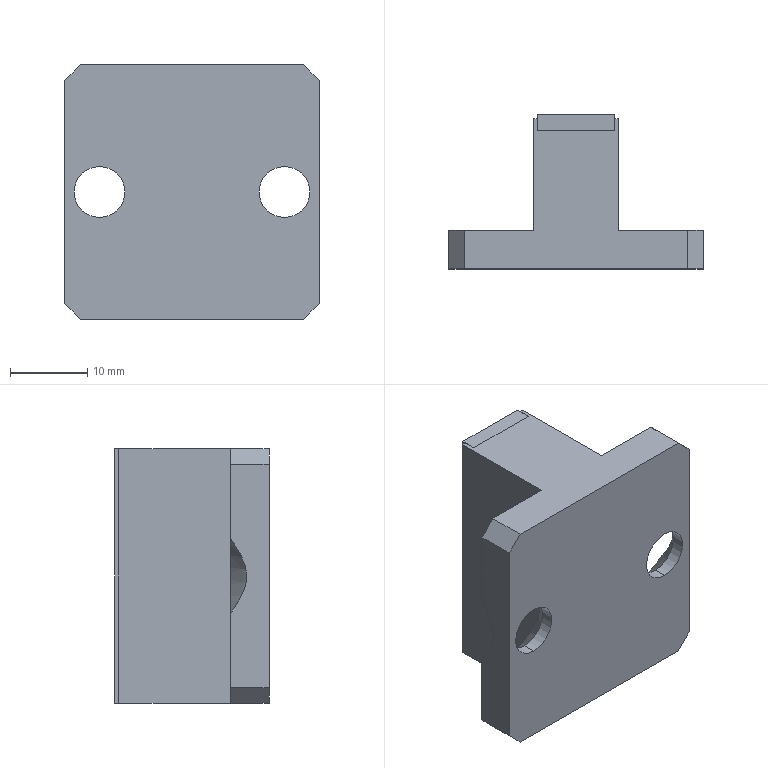Part | SolidWorks | features ICE 2, Chamfer 1, Extrusion 1, HoleWzd 1 | 2 solids | 36 faces | box 33 x 20 x 33 mm | volume 10213 mm3 | plane 28 | cylinder 4 | cone 4 | commonest cylinder face diameters 6.6 x4
STEP:
#1=CARTESIAN_POINT('',(-5.,18.,-16.5));
#2=VERTEX_POINT('',#1);
#3=CARTESIAN_POINT('',(-5.,18.,16.5));
#4=VERTEX_POINT('',#3);
#5=CARTESIAN_POINT('',(-5.,18.,-16.5));
#6=DIRECTION('',(0.,0.,1.));
#7=VECTOR('',#6,1000.);
#8=LINE('',#5,#7);
#9=EDGE_CURVE('',#2,#4,#8,.T.);
#10=ORIENTED_EDGE('',*,*,#9,.T.);
#11=CARTESIAN_POINT('',(-5.,20.,16.5));
#12=VERTEX_POINT('',#11);
#13=CARTESIAN_POINT('',(-5.,20.,16.5));
#14=DIRECTION('',(0.,-1.,0.));
#15=VECTOR('',#14,1000.);
#16=LINE('',#13,#15);
#17=EDGE_CURVE('',#12,#4,#16,.T.);
#18=ORIENTED_EDGE('',*,*,#17,.F.);
#19=CARTESIAN_POINT('',(-5.,20.,-16.5));
#20=VERTEX_POINT('',#19);
#21=CARTESIAN_POINT('',(-5.,20.,-16.5));
#22=DIRECTION('',(0.,0.,1.));
#23=VECTOR('',#22,1000.);
#24=LINE('',#21,#23);
#25=EDGE_CURVE('',#20,#12,#24,.T.);
#26=ORIENTED_EDGE('',*,*,#25,.F.);
#27=CARTESIAN_POINT('',(-5.,20.,-16.5));
#28=DIRECTION('',(0.,-1.,0.));
#29=VECTOR('',#28,1000.);
#30=LINE('',#27,#29);
#31=EDGE_CURVE('',#20,#2,#30,.T.);
#32=ORIENTED_EDGE('',*,*,#31,.T.);
#33=EDGE_LOOP('',(#10,#18,#26,#32));
#34=FACE_OUTER_BOUND('',#33,.T.);
#35=CARTESIAN_POINT('',(-5.,20.,-16.5));
#36=DIRECTION('',(1.,0.,0.));
#37=DIRECTION('',(0.,0.,-1.));
#38=AXIS2_PLACEMENT_3D('',#35,#36,#37);
#39=PLANE('',#38);
#40=ADVANCED_FACE('',(#34),#39,.F.);
#41=CARTESIAN_POINT('',(5.,18.,16.5));
#42=VERTEX_POINT('',#41);
#43=CARTESIAN_POINT('',(-5.,18.,16.5));
#44=DIRECTION('',(1.,0.,0.));
#45=VECTOR('',#44,1000.);
#46=LINE('',#43,#45);
#47=EDGE_CURVE('',#4,#42,#46,.T.);
#48=ORIENTED_EDGE('',*,*,#47,.T.);
#49=CARTESIAN_POINT('',(5.,20.,16.5));
#50=VERTEX_POINT('',#49);
#51=CARTESIAN_POINT('',(5.,20.,16.5));
#52=DIRECTION('',(0.,-1.,0.));
#53=VECTOR('',#52,1000.);
#54=LINE('',#51,#53);
#55=EDGE_CURVE('',#50,#42,#54,.T.);
#56=ORIENTED_EDGE('',*,*,#55,.F.);
#57=CARTESIAN_POINT('',(-5.,20.,16.5));
#58=DIRECTION('',(1.,0.,0.));
#59=VECTOR('',#58,1000.);
#60=LINE('',#57,#59);
#61=EDGE_CURVE('',#12,#50,#60,.T.);
#62=ORIENTED_EDGE('',*,*,#61,.F.);
#63=ORIENTED_EDGE('',*,*,#17,.T.);
#64=EDGE_LOOP('',(#48,#56,#62,#63));
#65=FACE_OUTER_BOUND('',#64,.T.);
#66=CARTESIAN_POINT('',(-5.,20.,16.5));
#67=DIRECTION('',(0.,0.,-1.));
#68=DIRECTION('',(-1.,0.,0.));
#69=AXIS2_PLACEMENT_3D('',#66,#67,#68);
#70=PLANE('',#69);
#71=ADVANCED_FACE('',(#65),#70,.F.);
#72=CARTESIAN_POINT('',(5.,18.,-16.5));
#73=VERTEX_POINT('',#72);
#74=CARTESIAN_POINT('',(5.,18.,-16.5));
#75=DIRECTION('',(0.,0.,-1.));
#76=VECTOR('',#75,1000.);
#77=LINE('',#74,#76);
#78=EDGE_CURVE('',#42,#73,#77,.T.);
#79=ORIENTED_EDGE('',*,*,#78,.T.);
#80=CARTESIAN_POINT('',(5.,20.,-16.5));
#81=VERTEX_POINT('',#80);
#82=CARTESIAN_POINT('',(5.,20.,-16.5));
#83=DIRECTION('',(0.,-1.,0.));
#84=VECTOR('',#83,1000.);
#85=LINE('',#82,#84);
#86=EDGE_CURVE('',#81,#73,#85,.T.);
#87=ORIENTED_EDGE('',*,*,#86,.F.);
#88=CARTESIAN_POINT('',(5.,20.,-16.5));
#89=DIRECTION('',(0.,0.,-1.));
#90=VECTOR('',#89,1000.);
#91=LINE('',#88,#90);
#92=EDGE_CURVE('',#50,#81,#91,.T.);
#93=ORIENTED_EDGE('',*,*,#92,.F.);
#94=ORIENTED_EDGE('',*,*,#55,.T.);
#95=EDGE_LOOP('',(#79,#87,#93,#94));
#96=FACE_OUTER_BOUND('',#95,.T.);
#97=CARTESIAN_POINT('',(5.,20.,-16.5));
#98=DIRECTION('',(-1.,0.,0.));
#99=DIRECTION('',(0.,0.,1.));
#100=AXIS2_PLACEMENT_3D('',#97,#98,#99);
#101=PLANE('',#100);
#102=ADVANCED_FACE('',(#96),#101,.F.);
#103=CARTESIAN_POINT('',(-5.,18.,-16.5));
#104=DIRECTION('',(-1.,0.,0.));
#105=VECTOR('',#104,1000.);
#106=LINE('',#103,#105);
#107=EDGE_CURVE('',#73,#2,#106,.T.);
#108=ORIENTED_EDGE('',*,*,#107,.T.);
#109=ORIENTED_EDGE('',*,*,#31,.F.);
#110=CARTESIAN_POINT('',(-5.,20.,-16.5));
#111=DIRECTION('',(-1.,0.,0.));
#112=VECTOR('',#111,1000.);
#113=LINE('',#110,#112);
#114=EDGE_CURVE('',#81,#20,#113,.T.);
#115=ORIENTED_EDGE('',*,*,#114,.F.);
#116=ORIENTED_EDGE('',*,*,#86,.T.);
#117=EDGE_LOOP('',(#108,#109,#115,#116));
#118=FACE_OUTER_BOUND('',#117,.T.);
#119=CARTESIAN_POINT('',(-5.,20.,-16.5));
#120=DIRECTION('',(0.,0.,1.));
#121=DIRECTION('',(1.,0.,0.));
#122=AXIS2_PLACEMENT_3D('',#119,#120,#121);
#123=PLANE('',#122);
#124=ADVANCED_FACE('',(#118),#123,.F.);
#125=ORIENTED_EDGE('',*,*,#25,.T.);
#126=ORIENTED_EDGE('',*,*,#61,.T.);
#127=ORIENTED_EDGE('',*,*,#92,.T.);
#128=ORIENTED_EDGE('',*,*,#114,.T.);
#129=EDGE_LOOP('',(#125,#126,#127,#128));
#130=FACE_OUTER_BOUND('',#129,.T.);
#131=CARTESIAN_POINT('',(-5.,20.,16.5));
#132=DIRECTION('',(0.,1.,0.));
#133=DIRECTION('',(0.,0.,1.));
#134=AXIS2_PLACEMENT_3D('',#131,#132,#133);
#135=PLANE('',#134);
#136=ADVANCED_FACE('',(#130),#135,.T.);
#137=ORIENTED_EDGE('',*,*,#9,.F.);
#138=ORIENTED_EDGE('',*,*,#107,.F.);
#139=ORIENTED_EDGE('',*,*,#78,.F.);
#140=ORIENTED_EDGE('',*,*,#47,.F.);
#141=EDGE_LOOP('',(#137,#138,#139,#140));
#142=FACE_OUTER_BOUND('',#141,.T.);
#143=CARTESIAN_POINT('',(-5.,18.,16.5));
#144=DIRECTION('',(0.,1.,0.));
#145=DIRECTION('',(0.,0.,1.));
#146=AXIS2_PLACEMENT_3D('',#143,#144,#145);
#147=PLANE('',#146);
#148=ADVANCED_FACE('',(#142),#147,.F.);
#149=CLOSED_SHELL('',(#40,#71,#102,#124,#136,#148));
#150=MANIFOLD_SOLID_BREP('',#149);
#151=CARTESIAN_POINT('',(-12.,0.,-3.3));
#152=VERTEX_POINT('',#151);
#153=CARTESIAN_POINT('',(-12.,0.,3.3));
#154=VERTEX_POINT('',#153);
#155=CARTESIAN_POINT('',(-12.,0.,0.));
#156=DIRECTION('',(0.,1.,0.));
#157=DIRECTION('',(0.,0.,1.));
#158=AXIS2_PLACEMENT_3D('',#155,#156,#157);
#159=CIRCLE('',#158,3.3);
#160=EDGE_CURVE('',#152,#154,#159,.T.);
#161=ORIENTED_EDGE('',*,*,#160,.F.);
#162=CARTESIAN_POINT('',(-12.,1.7,-3.3));
#163=VERTEX_POINT('',#162);
#164=CARTESIAN_POINT('',(-12.,5.,-3.3));
#165=DIRECTION('',(0.,1.,0.));
#166=VECTOR('',#165,1000.);
#167=LINE('',#164,#166);
#168=EDGE_CURVE('',#152,#163,#167,.T.);
#169=ORIENTED_EDGE('',*,*,#168,.T.);
#170=CARTESIAN_POINT('',(-12.,1.7,3.3));
#171=VERTEX_POINT('',#170);
#172=CARTESIAN_POINT('',(-12.,1.7,0.));
#173=DIRECTION('',(0.,1.,0.));
#174=DIRECTION('',(0.,0.,1.));
#175=AXIS2_PLACEMENT_3D('',#172,#173,#174);
#176=CIRCLE('',#175,3.3);
#177=EDGE_CURVE('',#163,#171,#176,.T.);
#178=ORIENTED_EDGE('',*,*,#177,.T.);
#179=CARTESIAN_POINT('',(-12.,5.,3.3));
#180=DIRECTION('',(0.,1.,0.));
#181=VECTOR('',#180,1000.);
#182=LINE('',#179,#181);
#183=EDGE_CURVE('',#154,#171,#182,.T.);
#184=ORIENTED_EDGE('',*,*,#183,.F.);
#185=EDGE_LOOP('',(#161,#169,#178,#184));
#186=FACE_OUTER_BOUND('',#185,.T.);
#187=CARTESIAN_POINT('',(-12.,5.,0.));
#188=DIRECTION('',(0.,1.,0.));
#189=DIRECTION('',(0.,0.,1.));
#190=AXIS2_PLACEMENT_3D('',#187,#188,#189);
#191=CYLINDRICAL_SURFACE('',#190,3.3);
#192=ADVANCED_FACE('',(#186),#191,.F.);
#193=ORIENTED_EDGE('',*,*,#177,.F.);
#194=CARTESIAN_POINT('',(-12.,5.,-6.6));
#195=VERTEX_POINT('',#194);
#196=CARTESIAN_POINT('',(-12.,5.,-6.6));
#197=DIRECTION('',(0.,0.7071,-0.7071));
#198=VECTOR('',#197,1000.);
#199=LINE('',#196,#198);
#200=EDGE_CURVE('',#163,#195,#199,.T.);
#201=ORIENTED_EDGE('',*,*,#200,.T.);
#202=CARTESIAN_POINT('',(-16.5,5.,-4.828));
#203=VERTEX_POINT('',#202);
#204=CARTESIAN_POINT('',(-12.,5.,0.));
#205=DIRECTION('',(0.,1.,0.));
#206=DIRECTION('',(0.,0.,1.));
#207=AXIS2_PLACEMENT_3D('',#204,#205,#206);
#208=CIRCLE('',#207,6.6);
#209=EDGE_CURVE('',#195,#203,#208,.T.);
#210=ORIENTED_EDGE('',*,*,#209,.T.);
#211=CARTESIAN_POINT('',(-16.5,5.,4.828));
#212=VERTEX_POINT('',#211);
#213=CARTESIAN_POINT('',(-16.5,5.,4.828));
#214=CARTESIAN_POINT('',(-16.5,4.737,4.469));
#215=CARTESIAN_POINT('',(-16.5,4.484,4.105));
#216=CARTESIAN_POINT('',(-16.5,4.007,3.358));
#217=CARTESIAN_POINT('',(-16.5,3.783,2.975));
#218=CARTESIAN_POINT('',(-16.5,3.487,2.378));
#219=CARTESIAN_POINT('',(-16.5,3.394,2.175));
#220=CARTESIAN_POINT('',(-16.5,3.228,1.758));
#221=CARTESIAN_POINT('',(-16.5,3.153,1.545));
#222=CARTESIAN_POINT('',(-16.5,3.032,1.115));
#223=CARTESIAN_POINT('',(-16.5,2.983,0.8975));
#224=CARTESIAN_POINT('',(-16.5,2.918,0.4556));
#225=CARTESIAN_POINT('',(-16.5,2.9,0.2295));
#226=CARTESIAN_POINT('',(-16.5,2.9,-0.4446));
#227=CARTESIAN_POINT('',(-16.5,2.967,-0.8847));
#228=CARTESIAN_POINT('',(-16.5,3.15,-1.534));
#229=CARTESIAN_POINT('',(-16.5,3.223,-1.747));
#230=CARTESIAN_POINT('',(-16.5,3.389,-2.162));
#231=CARTESIAN_POINT('',(-16.5,3.48,-2.364));
#232=CARTESIAN_POINT('',(-16.5,3.776,-2.962));
#233=CARTESIAN_POINT('',(-16.5,4.001,-3.347));
#234=CARTESIAN_POINT('',(-16.5,4.481,-4.1));
#235=CARTESIAN_POINT('',(-16.5,4.737,-4.468));
#236=CARTESIAN_POINT('',(-16.5,5.,-4.828));
#237=B_SPLINE_CURVE_WITH_KNOTS('',3,(#213,#214,#215,#216,#217,#218,#219,#220,#221,#222,#223,#224,#225,#226,#227,#228,#229,#230,#231,#232,#233,#234,#235,#236),.UNSPECIFIED.,.F.,.F.,(4,2,2,2,2,2,2,2,2,2,2,4),(0.01903,0.02036,0.02169,0.02236,0.02303,0.02369,0.02436,0.02569,0.02635,0.02702,0.02835,0.02968),.UNSPECIFIED.);
#238=EDGE_CURVE('',#212,#203,#237,.T.);
#239=ORIENTED_EDGE('',*,*,#238,.F.);
#240=CARTESIAN_POINT('',(-12.,5.,6.6));
#241=VERTEX_POINT('',#240);
#242=CARTESIAN_POINT('',(-12.,5.,0.));
#243=DIRECTION('',(0.,1.,0.));
#244=DIRECTION('',(0.,0.,1.));
#245=AXIS2_PLACEMENT_3D('',#242,#243,#244);
#246=CIRCLE('',#245,6.6);
#247=EDGE_CURVE('',#212,#241,#246,.T.);
#248=ORIENTED_EDGE('',*,*,#247,.T.);
#249=CARTESIAN_POINT('',(-12.,5.,6.6));
#250=DIRECTION('',(0.,0.7071,0.7071));
#251=VECTOR('',#250,1000.);
#252=LINE('',#249,#251);
#253=EDGE_CURVE('',#171,#241,#252,.T.);
#254=ORIENTED_EDGE('',*,*,#253,.F.);
#255=EDGE_LOOP('',(#193,#201,#210,#239,#248,#254));
#256=FACE_OUTER_BOUND('',#255,.T.);
#257=CARTESIAN_POINT('',(-12.,5.,0.));
#258=DIRECTION('',(0.,1.,0.));
#259=DIRECTION('',(0.,0.,1.));
#260=AXIS2_PLACEMENT_3D('',#257,#258,#259);
#261=CONICAL_SURFACE('',#260,6.6,0.7854);
#262=ADVANCED_FACE('',(#256),#261,.F.);
#263=CARTESIAN_POINT('',(12.,0.,-3.3));
#264=VERTEX_POINT('',#263);
#265=CARTESIAN_POINT('',(12.,0.,3.3));
#266=VERTEX_POINT('',#265);
#267=CARTESIAN_POINT('',(12.,0.,0.));
#268=DIRECTION('',(0.,1.,0.));
#269=DIRECTION('',(0.,0.,1.));
#270=AXIS2_PLACEMENT_3D('',#267,#268,#269);
#271=CIRCLE('',#270,3.3);
#272=EDGE_CURVE('',#264,#266,#271,.T.);
#273=ORIENTED_EDGE('',*,*,#272,.F.);
#274=CARTESIAN_POINT('',(12.,1.7,-3.3));
#275=VERTEX_POINT('',#274);
#276=CARTESIAN_POINT('',(12.,5.,-3.3));
#277=DIRECTION('',(0.,1.,0.));
#278=VECTOR('',#277,1000.);
#279=LINE('',#276,#278);
#280=EDGE_CURVE('',#264,#275,#279,.T.);
#281=ORIENTED_EDGE('',*,*,#280,.T.);
#282=CARTESIAN_POINT('',(12.,1.7,3.3));
#283=VERTEX_POINT('',#282);
#284=CARTESIAN_POINT('',(12.,1.7,0.));
#285=DIRECTION('',(0.,1.,0.));
#286=DIRECTION('',(0.,0.,1.));
#287=AXIS2_PLACEMENT_3D('',#284,#285,#286);
#288=CIRCLE('',#287,3.3);
#289=EDGE_CURVE('',#275,#283,#288,.T.);
#290=ORIENTED_EDGE('',*,*,#289,.T.);
#291=CARTESIAN_POINT('',(12.,5.,3.3));
#292=DIRECTION('',(0.,1.,0.));
#293=VECTOR('',#292,1000.);
#294=LINE('',#291,#293);
#295=EDGE_CURVE('',#266,#283,#294,.T.);
#296=ORIENTED_EDGE('',*,*,#295,.F.);
#297=EDGE_LOOP('',(#273,#281,#290,#296));
#298=FACE_OUTER_BOUND('',#297,.T.);
#299=CARTESIAN_POINT('',(12.,5.,0.));
#300=DIRECTION('',(0.,1.,0.));
#301=DIRECTION('',(0.,0.,1.));
#302=AXIS2_PLACEMENT_3D('',#299,#300,#301);
#303=CYLINDRICAL_SURFACE('',#302,3.3);
#304=ADVANCED_FACE('',(#298),#303,.F.);
#305=ORIENTED_EDGE('',*,*,#289,.F.);
#306=CARTESIAN_POINT('',(12.,5.,-6.6));
#307=VERTEX_POINT('',#306);
#308=CARTESIAN_POINT('',(12.,5.,-6.6));
#309=DIRECTION('',(0.,0.7071,-0.7071));
#310=VECTOR('',#309,1000.);
#311=LINE('',#308,#310);
#312=EDGE_CURVE('',#275,#307,#311,.T.);
#313=ORIENTED_EDGE('',*,*,#312,.T.);
#314=CARTESIAN_POINT('',(5.5,5.,-1.145));
#315=VERTEX_POINT('',#314);
#316=CARTESIAN_POINT('',(12.,5.,0.));
#317=DIRECTION('',(0.,1.,0.));
#318=DIRECTION('',(0.,0.,1.));
#319=AXIS2_PLACEMENT_3D('',#316,#317,#318);
#320=CIRCLE('',#319,6.6);
#321=EDGE_CURVE('',#307,#315,#320,.T.);
#322=ORIENTED_EDGE('',*,*,#321,.T.);
#323=CARTESIAN_POINT('',(5.5,5.,1.145));
#324=VERTEX_POINT('',#323);
#325=CARTESIAN_POINT('',(12.,5.,0.));
#326=DIRECTION('',(0.,1.,0.));
#327=DIRECTION('',(0.,0.,1.));
#328=AXIS2_PLACEMENT_3D('',#325,#326,#327);
#329=CIRCLE('',#328,6.6);
#330=EDGE_CURVE('',#315,#324,#329,.T.);
#331=ORIENTED_EDGE('',*,*,#330,.T.);
#332=CARTESIAN_POINT('',(12.,5.,6.6));
#333=VERTEX_POINT('',#332);
#334=CARTESIAN_POINT('',(12.,5.,0.));
#335=DIRECTION('',(0.,1.,0.));
#336=DIRECTION('',(0.,0.,1.));
#337=AXIS2_PLACEMENT_3D('',#334,#335,#336);
#338=CIRCLE('',#337,6.6);
#339=EDGE_CURVE('',#324,#333,#338,.T.);
#340=ORIENTED_EDGE('',*,*,#339,.T.);
#341=CARTESIAN_POINT('',(12.,5.,6.6));
#342=DIRECTION('',(0.,0.7071,0.7071));
#343=VECTOR('',#342,1000.);
#344=LINE('',#341,#343);
#345=EDGE_CURVE('',#283,#333,#344,.T.);
#346=ORIENTED_EDGE('',*,*,#345,.F.);
#347=EDGE_LOOP('',(#305,#313,#322,#331,#340,#346));
#348=FACE_OUTER_BOUND('',#347,.T.);
#349=CARTESIAN_POINT('',(12.,5.,0.));
#350=DIRECTION('',(0.,1.,0.));
#351=DIRECTION('',(0.,0.,1.));
#352=AXIS2_PLACEMENT_3D('',#349,#350,#351);
#353=CONICAL_SURFACE('',#352,6.6,0.7854);
#354=ADVANCED_FACE('',(#348),#353,.F.);
#355=CARTESIAN_POINT('',(-5.5,5.,-16.5));
#356=VERTEX_POINT('',#355);
#357=CARTESIAN_POINT('',(-14.5,5.,-16.5));
#358=VERTEX_POINT('',#357);
#359=CARTESIAN_POINT('',(-16.5,5.,-16.5));
#360=DIRECTION('',(-1.,0.,0.));
#361=VECTOR('',#360,1000.);
#362=LINE('',#359,#361);
#363=EDGE_CURVE('',#356,#358,#362,.T.);
#364=ORIENTED_EDGE('',*,*,#363,.T.);
#365=CARTESIAN_POINT('',(-16.5,5.,-14.5));
#366=VERTEX_POINT('',#365);
#367=CARTESIAN_POINT('',(-16.5,5.,-14.5));
#368=DIRECTION('',(-0.7071,0.,0.7071));
#369=VECTOR('',#368,1000.);
#370=LINE('',#367,#369);
#371=EDGE_CURVE('',#358,#366,#370,.T.);
#372=ORIENTED_EDGE('',*,*,#371,.T.);
#373=CARTESIAN_POINT('',(-16.5,5.,16.5));
#374=DIRECTION('',(0.,0.,-1.));
#375=VECTOR('',#374,1000.);
#376=LINE('',#373,#375);
#377=EDGE_CURVE('',#203,#366,#376,.T.);
#378=ORIENTED_EDGE('',*,*,#377,.F.);
#379=ORIENTED_EDGE('',*,*,#209,.F.);
#380=CARTESIAN_POINT('',(-5.5,5.,-1.145));
#381=VERTEX_POINT('',#380);
#382=CARTESIAN_POINT('',(-12.,5.,0.));
#383=DIRECTION('',(0.,1.,0.));
#384=DIRECTION('',(0.,0.,1.));
#385=AXIS2_PLACEMENT_3D('',#382,#383,#384);
#386=CIRCLE('',#385,6.6);
#387=EDGE_CURVE('',#381,#195,#386,.T.);
#388=ORIENTED_EDGE('',*,*,#387,.F.);
#389=CARTESIAN_POINT('',(-5.5,5.,16.5));
#390=DIRECTION('',(0.,0.,-1.));
#391=VECTOR('',#390,1000.);
#392=LINE('',#389,#391);
#393=EDGE_CURVE('',#381,#356,#392,.T.);
#394=ORIENTED_EDGE('',*,*,#393,.T.);
#395=EDGE_LOOP('',(#364,#372,#378,#379,#388,#394));
#396=FACE_OUTER_BOUND('',#395,.T.);
#397=CARTESIAN_POINT('',(-16.5,5.,16.5));
#398=DIRECTION('',(0.,-1.,0.));
#399=DIRECTION('',(1.,0.,0.));
#400=AXIS2_PLACEMENT_3D('',#397,#398,#399);
#401=PLANE('',#400);
#402=ADVANCED_FACE('',(#396),#401,.F.);
#403=CARTESIAN_POINT('',(-16.5,5.,14.5));
#404=VERTEX_POINT('',#403);
#405=CARTESIAN_POINT('',(-16.5,5.,16.5));
#406=DIRECTION('',(0.,0.,-1.));
#407=VECTOR('',#406,1000.);
#408=LINE('',#405,#407);
#409=EDGE_CURVE('',#404,#212,#408,.T.);
#410=ORIENTED_EDGE('',*,*,#409,.F.);
#411=CARTESIAN_POINT('',(-14.5,5.,16.5));
#412=VERTEX_POINT('',#411);
#413=CARTESIAN_POINT('',(-14.5,5.,16.5));
#414=DIRECTION('',(0.7071,0.,0.7071));
#415=VECTOR('',#414,1000.);
#416=LINE('',#413,#415);
#417=EDGE_CURVE('',#404,#412,#416,.T.);
#418=ORIENTED_EDGE('',*,*,#417,.T.);
#419=CARTESIAN_POINT('',(-5.5,5.,16.5));
#420=VERTEX_POINT('',#419);
#421=CARTESIAN_POINT('',(-16.5,5.,16.5));
#422=DIRECTION('',(-1.,0.,0.));
#423=VECTOR('',#422,1000.);
#424=LINE('',#421,#423);
#425=EDGE_CURVE('',#420,#412,#424,.T.);
#426=ORIENTED_EDGE('',*,*,#425,.F.);
#427=CARTESIAN_POINT('',(-5.5,5.,1.145));
#428=VERTEX_POINT('',#427);
#429=CARTESIAN_POINT('',(-5.5,5.,16.5));
#430=DIRECTION('',(0.,0.,-1.));
#431=VECTOR('',#430,1000.);
#432=LINE('',#429,#431);
#433=EDGE_CURVE('',#420,#428,#432,.T.);
#434=ORIENTED_EDGE('',*,*,#433,.T.);
#435=CARTESIAN_POINT('',(-12.,5.,0.));
#436=DIRECTION('',(0.,1.,0.));
#437=DIRECTION('',(0.,0.,1.));
#438=AXIS2_PLACEMENT_3D('',#435,#436,#437);
#439=CIRCLE('',#438,6.6);
#440=EDGE_CURVE('',#241,#428,#439,.T.);
#441=ORIENTED_EDGE('',*,*,#440,.F.);
#442=ORIENTED_EDGE('',*,*,#247,.F.);
#443=EDGE_LOOP('',(#410,#418,#426,#434,#441,#442));
#444=FACE_OUTER_BOUND('',#443,.T.);
#445=CARTESIAN_POINT('',(-16.5,5.,16.5));
#446=DIRECTION('',(0.,-1.,0.));
#447=DIRECTION('',(1.,0.,0.));
#448=AXIS2_PLACEMENT_3D('',#445,#446,#447);
#449=PLANE('',#448);
#450=ADVANCED_FACE('',(#444),#449,.F.);
#451=CARTESIAN_POINT('',(16.5,5.,-4.828));
#452=VERTEX_POINT('',#451);
#453=CARTESIAN_POINT('',(16.5,5.,-14.5));
#454=VERTEX_POINT('',#453);
#455=CARTESIAN_POINT('',(16.5,5.,16.5));
#456=DIRECTION('',(0.,0.,-1.));
#457=VECTOR('',#456,1000.);
#458=LINE('',#455,#457);
#459=EDGE_CURVE('',#452,#454,#458,.T.);
#460=ORIENTED_EDGE('',*,*,#459,.T.);
#461=CARTESIAN_POINT('',(14.5,5.,-16.5));
#462=VERTEX_POINT('',#461);
#463=CARTESIAN_POINT('',(16.5,5.,-14.5));
#464=DIRECTION('',(-0.7071,0.,-0.7071));
#465=VECTOR('',#464,1000.);
#466=LINE('',#463,#465);
#467=EDGE_CURVE('',#454,#462,#466,.T.);
#468=ORIENTED_EDGE('',*,*,#467,.T.);
#469=CARTESIAN_POINT('',(5.5,5.,-16.5));
#470=VERTEX_POINT('',#469);
#471=CARTESIAN_POINT('',(16.5,5.,-16.5));
#472=DIRECTION('',(-1.,0.,0.));
#473=VECTOR('',#472,1000.);
#474=LINE('',#471,#473);
#475=EDGE_CURVE('',#462,#470,#474,.T.);
#476=ORIENTED_EDGE('',*,*,#475,.T.);
#477=CARTESIAN_POINT('',(5.5,5.,16.5));
#478=DIRECTION('',(0.,0.,-1.));
#479=VECTOR('',#478,1000.);
#480=LINE('',#477,#479);
#481=EDGE_CURVE('',#315,#470,#480,.T.);
#482=ORIENTED_EDGE('',*,*,#481,.F.);
#483=ORIENTED_EDGE('',*,*,#321,.F.);
#484=CARTESIAN_POINT('',(12.,5.,0.));
#485=DIRECTION('',(0.,1.,0.));
#486=DIRECTION('',(0.,0.,1.));
#487=AXIS2_PLACEMENT_3D('',#484,#485,#486);
#488=CIRCLE('',#487,6.6);
#489=EDGE_CURVE('',#452,#307,#488,.T.);
#490=ORIENTED_EDGE('',*,*,#489,.F.);
#491=EDGE_LOOP('',(#460,#468,#476,#482,#483,#490));
#492=FACE_OUTER_BOUND('',#491,.T.);
#493=CARTESIAN_POINT('',(16.5,5.,16.5));
#494=DIRECTION('',(0.,-1.,0.));
#495=DIRECTION('',(1.,0.,0.));
#496=AXIS2_PLACEMENT_3D('',#493,#494,#495);
#497=PLANE('',#496);
#498=ADVANCED_FACE('',(#492),#497,.F.);
#499=CARTESIAN_POINT('',(14.5,5.,16.5));
#500=VERTEX_POINT('',#499);
#501=CARTESIAN_POINT('',(5.5,5.,16.5));
#502=VERTEX_POINT('',#501);
#503=CARTESIAN_POINT('',(16.5,5.,16.5));
#504=DIRECTION('',(-1.,0.,0.));
#505=VECTOR('',#504,1000.);
#506=LINE('',#503,#505);
#507=EDGE_CURVE('',#500,#502,#506,.T.);
#508=ORIENTED_EDGE('',*,*,#507,.F.);
#509=CARTESIAN_POINT('',(16.5,5.,14.5));
#510=VERTEX_POINT('',#509);
#511=CARTESIAN_POINT('',(14.5,5.,16.5));
#512=DIRECTION('',(0.7071,0.,-0.7071));
#513=VECTOR('',#512,1000.);
#514=LINE('',#511,#513);
#515=EDGE_CURVE('',#500,#510,#514,.T.);
#516=ORIENTED_EDGE('',*,*,#515,.T.);
#517=CARTESIAN_POINT('',(16.5,5.,4.828));
#518=VERTEX_POINT('',#517);
#519=CARTESIAN_POINT('',(16.5,5.,16.5));
#520=DIRECTION('',(0.,0.,-1.));
#521=VECTOR('',#520,1000.);
#522=LINE('',#519,#521);
#523=EDGE_CURVE('',#510,#518,#522,.T.);
#524=ORIENTED_EDGE('',*,*,#523,.T.);
#525=CARTESIAN_POINT('',(12.,5.,0.));
#526=DIRECTION('',(0.,1.,0.));
#527=DIRECTION('',(0.,0.,1.));
#528=AXIS2_PLACEMENT_3D('',#525,#526,#527);
#529=CIRCLE('',#528,6.6);
#530=EDGE_CURVE('',#333,#518,#529,.T.);
#531=ORIENTED_EDGE('',*,*,#530,.F.);
#532=ORIENTED_EDGE('',*,*,#339,.F.);
#533=CARTESIAN_POINT('',(5.5,5.,16.5));
#534=DIRECTION('',(0.,0.,-1.));
#535=VECTOR('',#534,1000.);
#536=LINE('',#533,#535);
#537=EDGE_CURVE('',#502,#324,#536,.T.);
#538=ORIENTED_EDGE('',*,*,#537,.F.);
#539=EDGE_LOOP('',(#508,#516,#524,#531,#532,#538));
#540=FACE_OUTER_BOUND('',#539,.T.);
#541=CARTESIAN_POINT('',(16.5,5.,16.5));
#542=DIRECTION('',(0.,-1.,0.));
#543=DIRECTION('',(1.,0.,0.));
#544=AXIS2_PLACEMENT_3D('',#541,#542,#543);
#545=PLANE('',#544);
#546=ADVANCED_FACE('',(#540),#545,.F.);
#547=CARTESIAN_POINT('',(-5.,19.5,16.5));
#548=VERTEX_POINT('',#547);
#549=CARTESIAN_POINT('',(-5.5,19.5,16.5));
#550=VERTEX_POINT('',#549);
#551=CARTESIAN_POINT('',(5.5,19.5,16.5));
#552=DIRECTION('',(-1.,0.,0.));
#553=VECTOR('',#552,1000.);
#554=LINE('',#551,#553);
#555=EDGE_CURVE('',#548,#550,#554,.T.);
#556=ORIENTED_EDGE('',*,*,#555,.F.);
#557=CARTESIAN_POINT('',(-5.,19.5,-16.5));
#558=VERTEX_POINT('',#557);
#559=CARTESIAN_POINT('',(-5.,19.5,-16.5));
#560=DIRECTION('',(0.,0.,1.));
#561=VECTOR('',#560,1000.);
#562=LINE('',#559,#561);
#563=EDGE_CURVE('',#558,#548,#562,.T.);
#564=ORIENTED_EDGE('',*,*,#563,.F.);
#565=CARTESIAN_POINT('',(-5.5,19.5,-16.5));
#566=VERTEX_POINT('',#565);
#567=CARTESIAN_POINT('',(5.5,19.5,-16.5));
#568=DIRECTION('',(-1.,0.,0.));
#569=VECTOR('',#568,1000.);
#570=LINE('',#567,#569);
#571=EDGE_CURVE('',#558,#566,#570,.T.);
#572=ORIENTED_EDGE('',*,*,#571,.T.);
#573=CARTESIAN_POINT('',(-5.5,19.5,16.5));
#574=DIRECTION('',(0.,0.,-1.));
#575=VECTOR('',#574,1000.);
#576=LINE('',#573,#575);
#577=EDGE_CURVE('',#550,#566,#576,.T.);
#578=ORIENTED_EDGE('',*,*,#577,.F.);
#579=EDGE_LOOP('',(#556,#564,#572,#578));
#580=FACE_OUTER_BOUND('',#579,.T.);
#581=CARTESIAN_POINT('',(5.5,19.5,16.5));
#582=DIRECTION('',(0.,-1.,0.));
#583=DIRECTION('',(0.,0.,-1.));
#584=AXIS2_PLACEMENT_3D('',#581,#582,#583);
#585=PLANE('',#584);
#586=ADVANCED_FACE('',(#580),#585,.F.);
#587=CARTESIAN_POINT('',(16.5,0.,14.5));
#588=VERTEX_POINT('',#587);
#589=CARTESIAN_POINT('',(16.5,0.,-14.5));
#590=VERTEX_POINT('',#589);
#591=CARTESIAN_POINT('',(16.5,0.,16.5));
#592=DIRECTION('',(0.,0.,-1.));
#593=VECTOR('',#592,1000.);
#594=LINE('',#591,#593);
#595=EDGE_CURVE('',#588,#590,#594,.T.);
#596=ORIENTED_EDGE('',*,*,#595,.T.);
#597=CARTESIAN_POINT('',(16.5,0.,-14.5));
#598=DIRECTION('',(0.,1.,0.));
#599=VECTOR('',#598,1000.);
#600=LINE('',#597,#599);
#601=EDGE_CURVE('',#590,#454,#600,.T.);
#602=ORIENTED_EDGE('',*,*,#601,.T.);
#603=ORIENTED_EDGE('',*,*,#459,.F.);
#604=CARTESIAN_POINT('',(16.5,5.,-4.828));
#605=CARTESIAN_POINT('',(16.5,4.737,-4.468));
#606=CARTESIAN_POINT('',(16.5,4.481,-4.1));
#607=CARTESIAN_POINT('',(16.5,4.001,-3.347));
#608=CARTESIAN_POINT('',(16.5,3.776,-2.962));
#609=CARTESIAN_POINT('',(16.5,3.48,-2.364));
#610=CARTESIAN_POINT('',(16.5,3.389,-2.162));
#611=CARTESIAN_POINT('',(16.5,3.223,-1.747));
#612=CARTESIAN_POINT('',(16.5,3.15,-1.534));
#613=CARTESIAN_POINT('',(16.5,2.967,-0.8847));
#614=CARTESIAN_POINT('',(16.5,2.9,-0.4446));
#615=CARTESIAN_POINT('',(16.5,2.9,0.2295));
#616=CARTESIAN_POINT('',(16.5,2.918,0.4556));
#617=CARTESIAN_POINT('',(16.5,2.983,0.8975));
#618=CARTESIAN_POINT('',(16.5,3.032,1.115));
#619=CARTESIAN_POINT('',(16.5,3.153,1.545));
#620=CARTESIAN_POINT('',(16.5,3.228,1.758));
#621=CARTESIAN_POINT('',(16.5,3.394,2.175));
#622=CARTESIAN_POINT('',(16.5,3.487,2.378));
#623=CARTESIAN_POINT('',(16.5,3.783,2.975));
#624=CARTESIAN_POINT('',(16.5,4.007,3.358));
#625=CARTESIAN_POINT('',(16.5,4.484,4.105));
#626=CARTESIAN_POINT('',(16.5,4.737,4.469));
#627=CARTESIAN_POINT('',(16.5,5.,4.828));
#628=B_SPLINE_CURVE_WITH_KNOTS('',3,(#604,#605,#606,#607,#608,#609,#610,#611,#612,#613,#614,#615,#616,#617,#618,#619,#620,#621,#622,#623,#624,#625,#626,#627),.UNSPECIFIED.,.F.,.F.,(4,2,2,2,2,2,2,2,2,2,2,4),(0.006025,0.007361,0.008697,0.009366,0.01003,0.01137,0.01204,0.01271,0.01337,0.01404,0.01538,0.01672),.UNSPECIFIED.);
#629=EDGE_CURVE('',#452,#518,#628,.T.);
#630=ORIENTED_EDGE('',*,*,#629,.T.);
#631=ORIENTED_EDGE('',*,*,#523,.F.);
#632=CARTESIAN_POINT('',(16.5,0.,14.5));
#633=DIRECTION('',(0.,-1.,0.));
#634=VECTOR('',#633,1000.);
#635=LINE('',#632,#634);
#636=EDGE_CURVE('',#510,#588,#635,.T.);
#637=ORIENTED_EDGE('',*,*,#636,.T.);
#638=EDGE_LOOP('',(#596,#602,#603,#630,#631,#637));
#639=FACE_OUTER_BOUND('',#638,.T.);
#640=CARTESIAN_POINT('',(16.5,0.,16.5));
#641=DIRECTION('',(-1.,0.,0.));
#642=DIRECTION('',(0.,0.,1.));
#643=AXIS2_PLACEMENT_3D('',#640,#641,#642);
#644=PLANE('',#643);
#645=ADVANCED_FACE('',(#639),#644,.F.);
#646=CARTESIAN_POINT('',(5.5,19.5,-16.5));
#647=VERTEX_POINT('',#646);
#648=CARTESIAN_POINT('',(5.5,19.5,-16.5));
#649=DIRECTION('',(0.,1.,0.));
#650=VECTOR('',#649,1000.);
#651=LINE('',#648,#650);
#652=EDGE_CURVE('',#470,#647,#651,.T.);
#653=ORIENTED_EDGE('',*,*,#652,.T.);
#654=CARTESIAN_POINT('',(5.5,19.5,16.5));
#655=VERTEX_POINT('',#654);
#656=CARTESIAN_POINT('',(5.5,19.5,16.5));
#657=DIRECTION('',(0.,0.,-1.));
#658=VECTOR('',#657,1000.);
#659=LINE('',#656,#658);
#660=EDGE_CURVE('',#655,#647,#659,.T.);
#661=ORIENTED_EDGE('',*,*,#660,.F.);
#662=CARTESIAN_POINT('',(5.5,19.5,16.5));
#663=DIRECTION('',(0.,1.,0.));
#664=VECTOR('',#663,1000.);
#665=LINE('',#662,#664);
#666=EDGE_CURVE('',#502,#655,#665,.T.);
#667=ORIENTED_EDGE('',*,*,#666,.F.);
#668=ORIENTED_EDGE('',*,*,#537,.T.);
#669=CARTESIAN_POINT('',(5.5,5.,16.5));
#670=DIRECTION('',(0.,0.,-1.));
#671=VECTOR('',#670,1000.);
#672=LINE('',#669,#671);
#673=EDGE_CURVE('',#324,#315,#672,.T.);
#674=ORIENTED_EDGE('',*,*,#673,.T.);
#675=ORIENTED_EDGE('',*,*,#481,.T.);
#676=EDGE_LOOP('',(#653,#661,#667,#668,#674,#675));
#677=FACE_OUTER_BOUND('',#676,.T.);
#678=CARTESIAN_POINT('',(5.5,19.5,16.5));
#679=DIRECTION('',(-1.,0.,0.));
#680=DIRECTION('',(0.,-1.,0.));
#681=AXIS2_PLACEMENT_3D('',#678,#679,#680);
#682=PLANE('',#681);
#683=ADVANCED_FACE('',(#677),#682,.F.);
#684=CARTESIAN_POINT('',(5.,19.5,-16.5));
#685=VERTEX_POINT('',#684);
#686=CARTESIAN_POINT('',(5.5,19.5,-16.5));
#687=DIRECTION('',(-1.,0.,0.));
#688=VECTOR('',#687,1000.);
#689=LINE('',#686,#688);
#690=EDGE_CURVE('',#647,#685,#689,.T.);
#691=ORIENTED_EDGE('',*,*,#690,.T.);
#692=CARTESIAN_POINT('',(5.,19.5,16.5));
#693=VERTEX_POINT('',#692);
#694=CARTESIAN_POINT('',(5.,19.5,-16.5));
#695=DIRECTION('',(0.,0.,1.));
#696=VECTOR('',#695,1000.);
#697=LINE('',#694,#696);
#698=EDGE_CURVE('',#685,#693,#697,.T.);
#699=ORIENTED_EDGE('',*,*,#698,.T.);
#700=CARTESIAN_POINT('',(5.5,19.5,16.5));
#701=DIRECTION('',(-1.,0.,0.));
#702=VECTOR('',#701,1000.);
#703=LINE('',#700,#702);
#704=EDGE_CURVE('',#655,#693,#703,.T.);
#705=ORIENTED_EDGE('',*,*,#704,.F.);
#706=ORIENTED_EDGE('',*,*,#660,.T.);
#707=EDGE_LOOP('',(#691,#699,#705,#706));
#708=FACE_OUTER_BOUND('',#707,.T.);
#709=CARTESIAN_POINT('',(5.5,19.5,16.5));
#710=DIRECTION('',(0.,-1.,0.));
#711=DIRECTION('',(0.,0.,-1.));
#712=AXIS2_PLACEMENT_3D('',#709,#710,#711);
#713=PLANE('',#712);
#714=ADVANCED_FACE('',(#708),#713,.F.);
#715=CARTESIAN_POINT('',(-5.5,19.5,-16.5));
#716=DIRECTION('',(0.,-1.,0.));
#717=VECTOR('',#716,1000.);
#718=LINE('',#715,#717);
#719=EDGE_CURVE('',#566,#356,#718,.T.);
#720=ORIENTED_EDGE('',*,*,#719,.T.);
#721=ORIENTED_EDGE('',*,*,#393,.F.);
#722=CARTESIAN_POINT('',(-5.5,5.,16.5));
#723=DIRECTION('',(0.,0.,-1.));
#724=VECTOR('',#723,1000.);
#725=LINE('',#722,#724);
#726=EDGE_CURVE('',#428,#381,#725,.T.);
#727=ORIENTED_EDGE('',*,*,#726,.F.);
#728=ORIENTED_EDGE('',*,*,#433,.F.);
#729=CARTESIAN_POINT('',(-5.5,19.5,16.5));
#730=DIRECTION('',(0.,-1.,0.));
#731=VECTOR('',#730,1000.);
#732=LINE('',#729,#731);
#733=EDGE_CURVE('',#550,#420,#732,.T.);
#734=ORIENTED_EDGE('',*,*,#733,.F.);
#735=ORIENTED_EDGE('',*,*,#577,.T.);
#736=EDGE_LOOP('',(#720,#721,#727,#728,#734,#735));
#737=FACE_OUTER_BOUND('',#736,.T.);
#738=CARTESIAN_POINT('',(-5.5,19.5,16.5));
#739=DIRECTION('',(1.,0.,0.));
#740=DIRECTION('',(0.,1.,0.));
#741=AXIS2_PLACEMENT_3D('',#738,#739,#740);
#742=PLANE('',#741);
#743=ADVANCED_FACE('',(#737),#742,.F.);
#744=CARTESIAN_POINT('',(-16.5,0.,14.5));
#745=VERTEX_POINT('',#744);
#746=CARTESIAN_POINT('',(-16.5,0.,-14.5));
#747=VERTEX_POINT('',#746);
#748=CARTESIAN_POINT('',(-16.5,0.,16.5));
#749=DIRECTION('',(0.,0.,-1.));
#750=VECTOR('',#749,1000.);
#751=LINE('',#748,#750);
#752=EDGE_CURVE('',#745,#747,#751,.T.);
#753=ORIENTED_EDGE('',*,*,#752,.F.);
#754=CARTESIAN_POINT('',(-16.5,5.,14.5));
#755=DIRECTION('',(0.,1.,0.));
#756=VECTOR('',#755,1000.);
#757=LINE('',#754,#756);
#758=EDGE_CURVE('',#745,#404,#757,.T.);
#759=ORIENTED_EDGE('',*,*,#758,.T.);
#760=ORIENTED_EDGE('',*,*,#409,.T.);
#761=ORIENTED_EDGE('',*,*,#238,.T.);
#762=ORIENTED_EDGE('',*,*,#377,.T.);
#763=CARTESIAN_POINT('',(-16.5,0.,-14.5));
#764=DIRECTION('',(0.,-1.,0.));
#765=VECTOR('',#764,1000.);
#766=LINE('',#763,#765);
#767=EDGE_CURVE('',#366,#747,#766,.T.);
#768=ORIENTED_EDGE('',*,*,#767,.T.);
#769=EDGE_LOOP('',(#753,#759,#760,#761,#762,#768));
#770=FACE_OUTER_BOUND('',#769,.T.);
#771=CARTESIAN_POINT('',(-16.5,0.,16.5));
#772=DIRECTION('',(1.,0.,0.));
#773=DIRECTION('',(0.,0.,-1.));
#774=AXIS2_PLACEMENT_3D('',#771,#772,#773);
#775=PLANE('',#774);
#776=ADVANCED_FACE('',(#770),#775,.F.);
#777=CARTESIAN_POINT('',(-12.,0.,0.));
#778=DIRECTION('',(0.,1.,0.));
#779=DIRECTION('',(0.,0.,1.));
#780=AXIS2_PLACEMENT_3D('',#777,#778,#779);
#781=CIRCLE('',#780,3.3);
#782=EDGE_CURVE('',#154,#152,#781,.T.);
#783=ORIENTED_EDGE('',*,*,#782,.T.);
#784=ORIENTED_EDGE('',*,*,#160,.T.);
#785=EDGE_LOOP('',(#783,#784));
#786=FACE_BOUND('',#785,.T.);
#787=CARTESIAN_POINT('',(12.,0.,0.));
#788=DIRECTION('',(0.,1.,0.));
#789=DIRECTION('',(0.,0.,1.));
#790=AXIS2_PLACEMENT_3D('',#787,#788,#789);
#791=CIRCLE('',#790,3.3);
#792=EDGE_CURVE('',#266,#264,#791,.T.);
#793=ORIENTED_EDGE('',*,*,#792,.T.);
#794=ORIENTED_EDGE('',*,*,#272,.T.);
#795=EDGE_LOOP('',(#793,#794));
#796=FACE_BOUND('',#795,.T.);
#797=CARTESIAN_POINT('',(-14.5,0.,-16.5));
#798=VERTEX_POINT('',#797);
#799=CARTESIAN_POINT('',(14.5,0.,-16.5));
#800=VERTEX_POINT('',#799);
#801=CARTESIAN_POINT('',(16.5,0.,-16.5));
#802=DIRECTION('',(1.,0.,0.));
#803=VECTOR('',#802,1000.);
#804=LINE('',#801,#803);
#805=EDGE_CURVE('',#798,#800,#804,.T.);
#806=ORIENTED_EDGE('',*,*,#805,.T.);
#807=CARTESIAN_POINT('',(16.5,0.,-14.5));
#808=DIRECTION('',(0.7071,0.,0.7071));
#809=VECTOR('',#808,1000.);
#810=LINE('',#807,#809);
#811=EDGE_CURVE('',#800,#590,#810,.T.);
#812=ORIENTED_EDGE('',*,*,#811,.T.);
#813=ORIENTED_EDGE('',*,*,#595,.F.);
#814=CARTESIAN_POINT('',(14.5,0.,16.5));
#815=VERTEX_POINT('',#814);
#816=CARTESIAN_POINT('',(14.5,0.,16.5));
#817=DIRECTION('',(-0.7071,0.,0.7071));
#818=VECTOR('',#817,1000.);
#819=LINE('',#816,#818);
#820=EDGE_CURVE('',#588,#815,#819,.T.);
#821=ORIENTED_EDGE('',*,*,#820,.T.);
#822=CARTESIAN_POINT('',(-14.5,0.,16.5));
#823=VERTEX_POINT('',#822);
#824=CARTESIAN_POINT('',(16.5,0.,16.5));
#825=DIRECTION('',(1.,0.,0.));
#826=VECTOR('',#825,1000.);
#827=LINE('',#824,#826);
#828=EDGE_CURVE('',#823,#815,#827,.T.);
#829=ORIENTED_EDGE('',*,*,#828,.F.);
#830=CARTESIAN_POINT('',(-14.5,0.,16.5));
#831=DIRECTION('',(-0.7071,0.,-0.7071));
#832=VECTOR('',#831,1000.);
#833=LINE('',#830,#832);
#834=EDGE_CURVE('',#823,#745,#833,.T.);
#835=ORIENTED_EDGE('',*,*,#834,.T.);
#836=ORIENTED_EDGE('',*,*,#752,.T.);
#837=CARTESIAN_POINT('',(-16.5,0.,-14.5));
#838=DIRECTION('',(0.7071,0.,-0.7071));
#839=VECTOR('',#838,1000.);
#840=LINE('',#837,#839);
#841=EDGE_CURVE('',#747,#798,#840,.T.);
#842=ORIENTED_EDGE('',*,*,#841,.T.);
#843=EDGE_LOOP('',(#806,#812,#813,#821,#829,#835,#836,#842));
#844=FACE_OUTER_BOUND('',#843,.T.);
#845=CARTESIAN_POINT('',(16.5,0.,16.5));
#846=DIRECTION('',(0.,1.,0.));
#847=DIRECTION('',(0.,0.,1.));
#848=AXIS2_PLACEMENT_3D('',#845,#846,#847);
#849=PLANE('',#848);
#850=ADVANCED_FACE('',(#786,#796,#844),#849,.F.);
#851=ORIENTED_EDGE('',*,*,#828,.T.);
#852=CARTESIAN_POINT('',(14.5,5.,16.5));
#853=DIRECTION('',(0.,1.,0.));
#854=VECTOR('',#853,1000.);
#855=LINE('',#852,#854);
#856=EDGE_CURVE('',#815,#500,#855,.T.);
#857=ORIENTED_EDGE('',*,*,#856,.T.);
#858=ORIENTED_EDGE('',*,*,#507,.T.);
#859=ORIENTED_EDGE('',*,*,#666,.T.);
#860=ORIENTED_EDGE('',*,*,#704,.T.);
#861=CARTESIAN_POINT('',(5.,18.,16.5));
#862=VERTEX_POINT('',#861);
#863=CARTESIAN_POINT('',(5.,19.5,16.5));
#864=DIRECTION('',(0.,1.,0.));
#865=VECTOR('',#864,1000.);
#866=LINE('',#863,#865);
#867=EDGE_CURVE('',#862,#693,#866,.T.);
#868=ORIENTED_EDGE('',*,*,#867,.F.);
#869=CARTESIAN_POINT('',(-5.,18.,16.5));
#870=VERTEX_POINT('',#869);
#871=CARTESIAN_POINT('',(-5.,18.,16.5));
#872=DIRECTION('',(1.,0.,0.));
#873=VECTOR('',#872,1000.);
#874=LINE('',#871,#873);
#875=EDGE_CURVE('',#870,#862,#874,.T.);
#876=ORIENTED_EDGE('',*,*,#875,.F.);
#877=CARTESIAN_POINT('',(-5.,19.5,16.5));
#878=DIRECTION('',(0.,-1.,0.));
#879=VECTOR('',#878,1000.);
#880=LINE('',#877,#879);
#881=EDGE_CURVE('',#548,#870,#880,.T.);
#882=ORIENTED_EDGE('',*,*,#881,.F.);
#883=ORIENTED_EDGE('',*,*,#555,.T.);
#884=ORIENTED_EDGE('',*,*,#733,.T.);
#885=ORIENTED_EDGE('',*,*,#425,.T.);
#886=CARTESIAN_POINT('',(-14.5,0.,16.5));
#887=DIRECTION('',(0.,-1.,0.));
#888=VECTOR('',#887,1000.);
#889=LINE('',#886,#888);
#890=EDGE_CURVE('',#412,#823,#889,.T.);
#891=ORIENTED_EDGE('',*,*,#890,.T.);
#892=EDGE_LOOP('',(#851,#857,#858,#859,#860,#868,#876,#882,#883,#884,#885,#891));
#893=FACE_OUTER_BOUND('',#892,.T.);
#894=CARTESIAN_POINT('',(16.5,5.,16.5));
#895=DIRECTION('',(0.,0.,1.));
#896=DIRECTION('',(1.,0.,0.));
#897=AXIS2_PLACEMENT_3D('',#894,#895,#896);
#898=PLANE('',#897);
#899=ADVANCED_FACE('',(#893),#898,.T.);
#900=ORIENTED_EDGE('',*,*,#475,.F.);
#901=CARTESIAN_POINT('',(14.5,5.,-16.5));
#902=DIRECTION('',(0.,-1.,0.));
#903=VECTOR('',#902,1000.);
#904=LINE('',#901,#903);
#905=EDGE_CURVE('',#462,#800,#904,.T.);
#906=ORIENTED_EDGE('',*,*,#905,.T.);
#907=ORIENTED_EDGE('',*,*,#805,.F.);
#908=CARTESIAN_POINT('',(-14.5,5.,-16.5));
#909=DIRECTION('',(0.,1.,0.));
#910=VECTOR('',#909,1000.);
#911=LINE('',#908,#910);
#912=EDGE_CURVE('',#798,#358,#911,.T.);
#913=ORIENTED_EDGE('',*,*,#912,.T.);
#914=ORIENTED_EDGE('',*,*,#363,.F.);
#915=ORIENTED_EDGE('',*,*,#719,.F.);
#916=ORIENTED_EDGE('',*,*,#571,.F.);
#917=CARTESIAN_POINT('',(-5.,18.,-16.5));
#918=VERTEX_POINT('',#917);
#919=CARTESIAN_POINT('',(-5.,19.5,-16.5));
#920=DIRECTION('',(0.,-1.,0.));
#921=VECTOR('',#920,1000.);
#922=LINE('',#919,#921);
#923=EDGE_CURVE('',#558,#918,#922,.T.);
#924=ORIENTED_EDGE('',*,*,#923,.T.);
#925=CARTESIAN_POINT('',(5.,18.,-16.5));
#926=VERTEX_POINT('',#925);
#927=CARTESIAN_POINT('',(-5.,18.,-16.5));
#928=DIRECTION('',(1.,0.,0.));
#929=VECTOR('',#928,1000.);
#930=LINE('',#927,#929);
#931=EDGE_CURVE('',#918,#926,#930,.T.);
#932=ORIENTED_EDGE('',*,*,#931,.T.);
#933=CARTESIAN_POINT('',(5.,19.5,-16.5));
#934=DIRECTION('',(0.,1.,0.));
#935=VECTOR('',#934,1000.);
#936=LINE('',#933,#935);
#937=EDGE_CURVE('',#926,#685,#936,.T.);
#938=ORIENTED_EDGE('',*,*,#937,.T.);
#939=ORIENTED_EDGE('',*,*,#690,.F.);
#940=ORIENTED_EDGE('',*,*,#652,.F.);
#941=EDGE_LOOP('',(#900,#906,#907,#913,#914,#915,#916,#924,#932,#938,#939,#940));
#942=FACE_OUTER_BOUND('',#941,.T.);
#943=CARTESIAN_POINT('',(16.5,5.,-16.5));
#944=DIRECTION('',(0.,0.,1.));
#945=DIRECTION('',(1.,0.,0.));
#946=AXIS2_PLACEMENT_3D('',#943,#944,#945);
#947=PLANE('',#946);
#948=ADVANCED_FACE('',(#942),#947,.F.);
#949=ORIENTED_EDGE('',*,*,#881,.T.);
#950=CARTESIAN_POINT('',(-5.,18.,-16.5));
#951=DIRECTION('',(0.,0.,1.));
#952=VECTOR('',#951,1000.);
#953=LINE('',#950,#952);
#954=EDGE_CURVE('',#918,#870,#953,.T.);
#955=ORIENTED_EDGE('',*,*,#954,.F.);
#956=ORIENTED_EDGE('',*,*,#923,.F.);
#957=ORIENTED_EDGE('',*,*,#563,.T.);
#958=EDGE_LOOP('',(#949,#955,#956,#957));
#959=FACE_OUTER_BOUND('',#958,.T.);
#960=CARTESIAN_POINT('',(-5.,19.5,-16.5));
#961=DIRECTION('',(-1.,0.,0.));
#962=DIRECTION('',(0.,-1.,0.));
#963=AXIS2_PLACEMENT_3D('',#960,#961,#962);
#964=PLANE('',#963);
#965=ADVANCED_FACE('',(#959),#964,.F.);
#966=ORIENTED_EDGE('',*,*,#867,.T.);
#967=ORIENTED_EDGE('',*,*,#698,.F.);
#968=ORIENTED_EDGE('',*,*,#937,.F.);
#969=CARTESIAN_POINT('',(5.,18.,-16.5));
#970=DIRECTION('',(0.,0.,1.));
#971=VECTOR('',#970,1000.);
#972=LINE('',#969,#971);
#973=EDGE_CURVE('',#926,#862,#972,.T.);
#974=ORIENTED_EDGE('',*,*,#973,.T.);
#975=EDGE_LOOP('',(#966,#967,#968,#974));
#976=FACE_OUTER_BOUND('',#975,.T.);
#977=CARTESIAN_POINT('',(5.,19.5,-16.5));
#978=DIRECTION('',(1.,0.,0.));
#979=DIRECTION('',(0.,1.,0.));
#980=AXIS2_PLACEMENT_3D('',#977,#978,#979);
#981=PLANE('',#980);
#982=ADVANCED_FACE('',(#976),#981,.F.);
#983=ORIENTED_EDGE('',*,*,#875,.T.);
#984=ORIENTED_EDGE('',*,*,#973,.F.);
#985=ORIENTED_EDGE('',*,*,#931,.F.);
#986=ORIENTED_EDGE('',*,*,#954,.T.);
#987=EDGE_LOOP('',(#983,#984,#985,#986));
#988=FACE_OUTER_BOUND('',#987,.T.);
#989=CARTESIAN_POINT('',(-5.,18.,-16.5));
#990=DIRECTION('',(0.,-1.,0.));
#991=DIRECTION('',(1.,0.,0.));
#992=AXIS2_PLACEMENT_3D('',#989,#990,#991);
#993=PLANE('',#992);
#994=ADVANCED_FACE('',(#988),#993,.F.);
#995=ORIENTED_EDGE('',*,*,#330,.F.);
#996=ORIENTED_EDGE('',*,*,#673,.F.);
#997=EDGE_LOOP('',(#995,#996));
#998=FACE_OUTER_BOUND('',#997,.T.);
#999=CARTESIAN_POINT('',(18.6,5.,0.));
#1000=DIRECTION('',(0.,1.,0.));
#1001=DIRECTION('',(0.,0.,1.));
#1002=AXIS2_PLACEMENT_3D('',#999,#1000,#1001);
#1003=PLANE('',#1002);
#1004=ADVANCED_FACE('',(#998),#1003,.F.);
#1005=ORIENTED_EDGE('',*,*,#312,.F.);
#1006=CARTESIAN_POINT('',(12.,1.7,0.));
#1007=DIRECTION('',(0.,1.,0.));
#1008=DIRECTION('',(0.,0.,1.));
#1009=AXIS2_PLACEMENT_3D('',#1006,#1007,#1008);
#1010=CIRCLE('',#1009,3.3);
#1011=EDGE_CURVE('',#283,#275,#1010,.T.);
#1012=ORIENTED_EDGE('',*,*,#1011,.F.);
#1013=ORIENTED_EDGE('',*,*,#345,.T.);
#1014=ORIENTED_EDGE('',*,*,#530,.T.);
#1015=ORIENTED_EDGE('',*,*,#629,.F.);
#1016=ORIENTED_EDGE('',*,*,#489,.T.);
#1017=EDGE_LOOP('',(#1005,#1012,#1013,#1014,#1015,#1016));
#1018=FACE_OUTER_BOUND('',#1017,.T.);
#1019=CARTESIAN_POINT('',(12.,5.,0.));
#1020=DIRECTION('',(0.,1.,0.));
#1021=DIRECTION('',(0.,0.,1.));
#1022=AXIS2_PLACEMENT_3D('',#1019,#1020,#1021);
#1023=CONICAL_SURFACE('',#1022,6.6,0.7854);
#1024=ADVANCED_FACE('',(#1018),#1023,.F.);
#1025=ORIENTED_EDGE('',*,*,#280,.F.);
#1026=ORIENTED_EDGE('',*,*,#792,.F.);
#1027=ORIENTED_EDGE('',*,*,#295,.T.);
#1028=ORIENTED_EDGE('',*,*,#1011,.T.);
#1029=EDGE_LOOP('',(#1025,#1026,#1027,#1028));
#1030=FACE_OUTER_BOUND('',#1029,.T.);
#1031=CARTESIAN_POINT('',(12.,5.,0.));
#1032=DIRECTION('',(0.,1.,0.));
#1033=DIRECTION('',(0.,0.,1.));
#1034=AXIS2_PLACEMENT_3D('',#1031,#1032,#1033);
#1035=CYLINDRICAL_SURFACE('',#1034,3.3);
#1036=ADVANCED_FACE('',(#1030),#1035,.F.);
#1037=ORIENTED_EDGE('',*,*,#726,.T.);
#1038=CARTESIAN_POINT('',(-12.,5.,0.));
#1039=DIRECTION('',(0.,1.,0.));
#1040=DIRECTION('',(0.,0.,1.));
#1041=AXIS2_PLACEMENT_3D('',#1038,#1039,#1040);
#1042=CIRCLE('',#1041,6.6);
#1043=EDGE_CURVE('',#428,#381,#1042,.T.);
#1044=ORIENTED_EDGE('',*,*,#1043,.F.);
#1045=EDGE_LOOP('',(#1037,#1044));
#1046=FACE_OUTER_BOUND('',#1045,.T.);
#1047=CARTESIAN_POINT('',(-5.4,5.,0.));
#1048=DIRECTION('',(0.,1.,0.));
#1049=DIRECTION('',(0.,0.,1.));
#1050=AXIS2_PLACEMENT_3D('',#1047,#1048,#1049);
#1051=PLANE('',#1050);
#1052=ADVANCED_FACE('',(#1046),#1051,.F.);
#1053=ORIENTED_EDGE('',*,*,#200,.F.);
#1054=CARTESIAN_POINT('',(-12.,1.7,0.));
#1055=DIRECTION('',(0.,1.,0.));
#1056=DIRECTION('',(0.,0.,1.));
#1057=AXIS2_PLACEMENT_3D('',#1054,#1055,#1056);
#1058=CIRCLE('',#1057,3.3);
#1059=EDGE_CURVE('',#171,#163,#1058,.T.);
#1060=ORIENTED_EDGE('',*,*,#1059,.F.);
#1061=ORIENTED_EDGE('',*,*,#253,.T.);
#1062=ORIENTED_EDGE('',*,*,#440,.T.);
#1063=ORIENTED_EDGE('',*,*,#1043,.T.);
#1064=ORIENTED_EDGE('',*,*,#387,.T.);
#1065=EDGE_LOOP('',(#1053,#1060,#1061,#1062,#1063,#1064));
#1066=FACE_OUTER_BOUND('',#1065,.T.);
#1067=CARTESIAN_POINT('',(-12.,5.,0.));
#1068=DIRECTION('',(0.,1.,0.));
#1069=DIRECTION('',(0.,0.,1.));
#1070=AXIS2_PLACEMENT_3D('',#1067,#1068,#1069);
#1071=CONICAL_SURFACE('',#1070,6.6,0.7854);
#1072=ADVANCED_FACE('',(#1066),#1071,.F.);
#1073=ORIENTED_EDGE('',*,*,#168,.F.);
#1074=ORIENTED_EDGE('',*,*,#782,.F.);
#1075=ORIENTED_EDGE('',*,*,#183,.T.);
#1076=ORIENTED_EDGE('',*,*,#1059,.T.);
#1077=EDGE_LOOP('',(#1073,#1074,#1075,#1076));
#1078=FACE_OUTER_BOUND('',#1077,.T.);
#1079=CARTESIAN_POINT('',(-12.,5.,0.));
#1080=DIRECTION('',(0.,1.,0.));
#1081=DIRECTION('',(0.,0.,1.));
#1082=AXIS2_PLACEMENT_3D('',#1079,#1080,#1081);
#1083=CYLINDRICAL_SURFACE('',#1082,3.3);
#1084=ADVANCED_FACE('',(#1078),#1083,.F.);
#1085=ORIENTED_EDGE('',*,*,#811,.F.);
#1086=ORIENTED_EDGE('',*,*,#905,.F.);
#1087=ORIENTED_EDGE('',*,*,#467,.F.);
#1088=ORIENTED_EDGE('',*,*,#601,.F.);
#1089=EDGE_LOOP('',(#1085,#1086,#1087,#1088));
#1090=FACE_OUTER_BOUND('',#1089,.T.);
#1091=CARTESIAN_POINT('',(16.5,0.,-14.5));
#1092=DIRECTION('',(-0.7071,0.,0.7071));
#1093=DIRECTION('',(0.7071,0.,0.7071));
#1094=AXIS2_PLACEMENT_3D('',#1091,#1092,#1093);
#1095=PLANE('',#1094);
#1096=ADVANCED_FACE('',(#1090),#1095,.F.);
#1097=ORIENTED_EDGE('',*,*,#820,.F.);
#1098=ORIENTED_EDGE('',*,*,#636,.F.);
#1099=ORIENTED_EDGE('',*,*,#515,.F.);
#1100=ORIENTED_EDGE('',*,*,#856,.F.);
#1101=EDGE_LOOP('',(#1097,#1098,#1099,#1100));
#1102=FACE_OUTER_BOUND('',#1101,.T.);
#1103=CARTESIAN_POINT('',(14.5,5.,16.5));
#1104=DIRECTION('',(0.7071,0.,0.7071));
#1105=DIRECTION('',(0.7071,0.,-0.7071));
#1106=AXIS2_PLACEMENT_3D('',#1103,#1104,#1105);
#1107=PLANE('',#1106);
#1108=ADVANCED_FACE('',(#1102),#1107,.T.);
#1109=ORIENTED_EDGE('',*,*,#417,.F.);
#1110=ORIENTED_EDGE('',*,*,#758,.F.);
#1111=ORIENTED_EDGE('',*,*,#834,.F.);
#1112=ORIENTED_EDGE('',*,*,#890,.F.);
#1113=EDGE_LOOP('',(#1109,#1110,#1111,#1112));
#1114=FACE_OUTER_BOUND('',#1113,.T.);
#1115=CARTESIAN_POINT('',(-14.5,5.,16.5));
#1116=DIRECTION('',(-0.7071,0.,0.7071));
#1117=DIRECTION('',(0.7071,0.,0.7071));
#1118=AXIS2_PLACEMENT_3D('',#1115,#1116,#1117);
#1119=PLANE('',#1118);
#1120=ADVANCED_FACE('',(#1114),#1119,.T.);
#1121=ORIENTED_EDGE('',*,*,#371,.F.);
#1122=ORIENTED_EDGE('',*,*,#912,.F.);
#1123=ORIENTED_EDGE('',*,*,#841,.F.);
#1124=ORIENTED_EDGE('',*,*,#767,.F.);
#1125=EDGE_LOOP('',(#1121,#1122,#1123,#1124));
#1126=FACE_OUTER_BOUND('',#1125,.T.);
#1127=CARTESIAN_POINT('',(-16.5,0.,-14.5));
#1128=DIRECTION('',(0.7071,0.,0.7071));
#1129=DIRECTION('',(0.7071,0.,-0.7071));
#1130=AXIS2_PLACEMENT_3D('',#1127,#1128,#1129);
#1131=PLANE('',#1130);
#1132=ADVANCED_FACE('',(#1126),#1131,.F.);
#1133=CLOSED_SHELL('',(#192,#262,#304,#354,#402,#450,#498,#546,#586,#645,#683,#714,#743,#776,#850,#899,#948,#965,#982,#994,#1004,#1024,#1036,#1052,#1072,#1084,#1096,#1108,#1120,#1132));
#1134=MANIFOLD_SOLID_BREP('',#1133);
#1135=CARTESIAN_POINT('',(0.,0.,0.));
#1136=DIRECTION('',(0.,0.,1.));
#1137=DIRECTION('',(1.,0.,0.));
#1138=AXIS2_PLACEMENT_3D('',#1135,#1136,#1137);
#1139=(LENGTH_UNIT()NAMED_UNIT(*)SI_UNIT(.MILLI.,.METRE.));
#1140=UNCERTAINTY_MEASURE_WITH_UNIT(LENGTH_MEASURE(0.00001),#1139,'','');
#1141=(NAMED_UNIT(*)PLANE_ANGLE_UNIT()SI_UNIT($,.RADIAN.));
#1142=(NAMED_UNIT(*)SI_UNIT($,.STERADIAN.)SOLID_ANGLE_UNIT());
#1143=(GEOMETRIC_REPRESENTATION_CONTEXT(3)GLOBAL_UNCERTAINTY_ASSIGNED_CONTEXT((#1140))GLOBAL_UNIT_ASSIGNED_CONTEXT((#1139,#1141,#1142))REPRESENTATION_CONTEXT('',''));
#1144=ADVANCED_BREP_SHAPE_REPRESENTATION('',(#150,#1134,#1138),#1143);